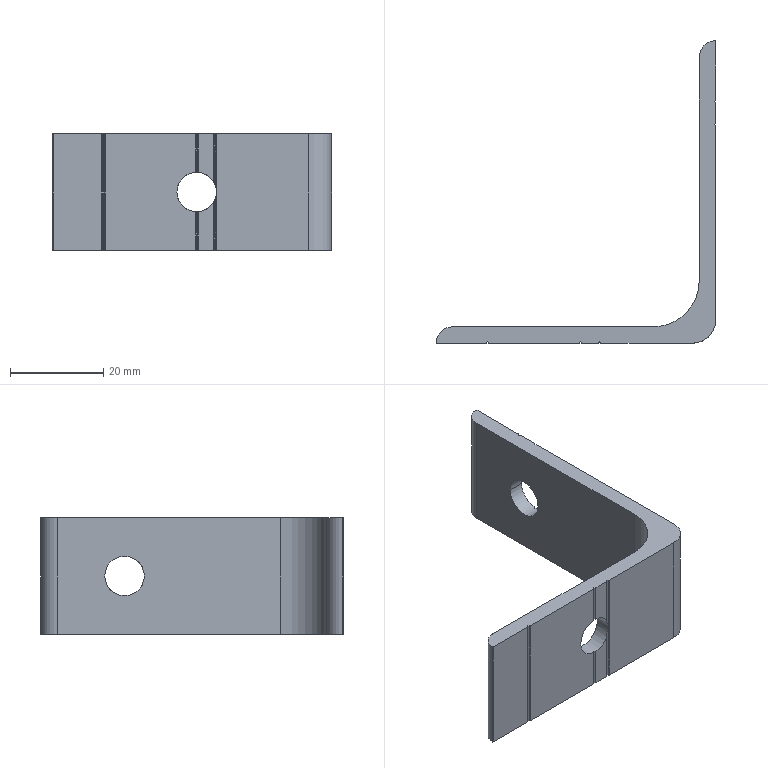Part | STEP file | 31E-01029QY13 | 1 solid | 53 faces | box 60 x 64.996 x 25 mm | volume 10496 mm3 | plane 27 | cylinder 26 | commonest cylinder face diameters 0.2 x15 8.5 x4 0.4 x3 7 x2 10 x1 20 x1